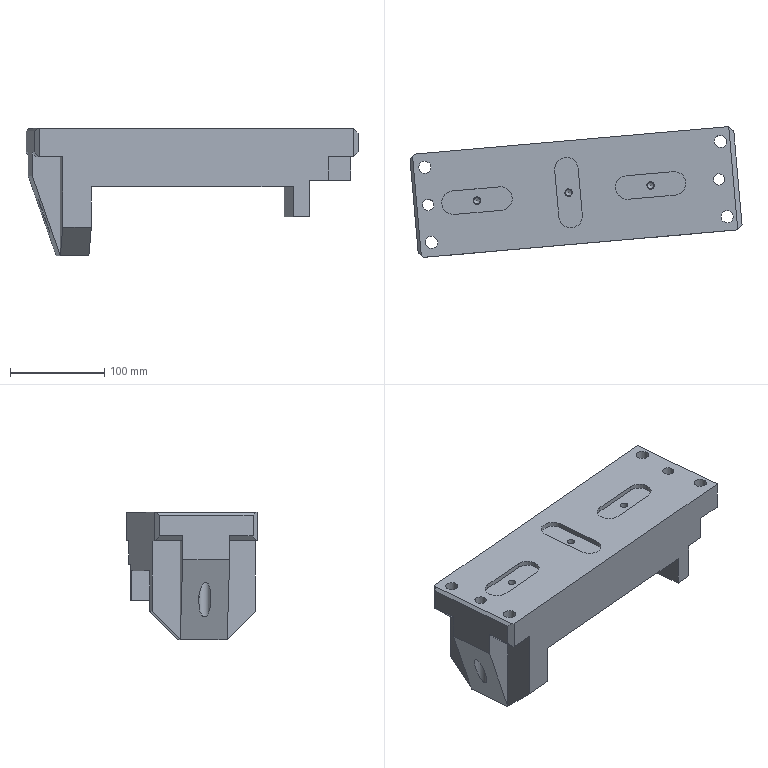Part | NX | features solid 2 | 1 solid | 82 faces | box 352.403 x 138.779 x 135 mm | volume 2442491 mm3 | plane 55 | cylinder 24 | cone 3 | commonest cylinder face diameters 13 x6 25 x6 20 x4 6.8 x3 8 x3 12 x2